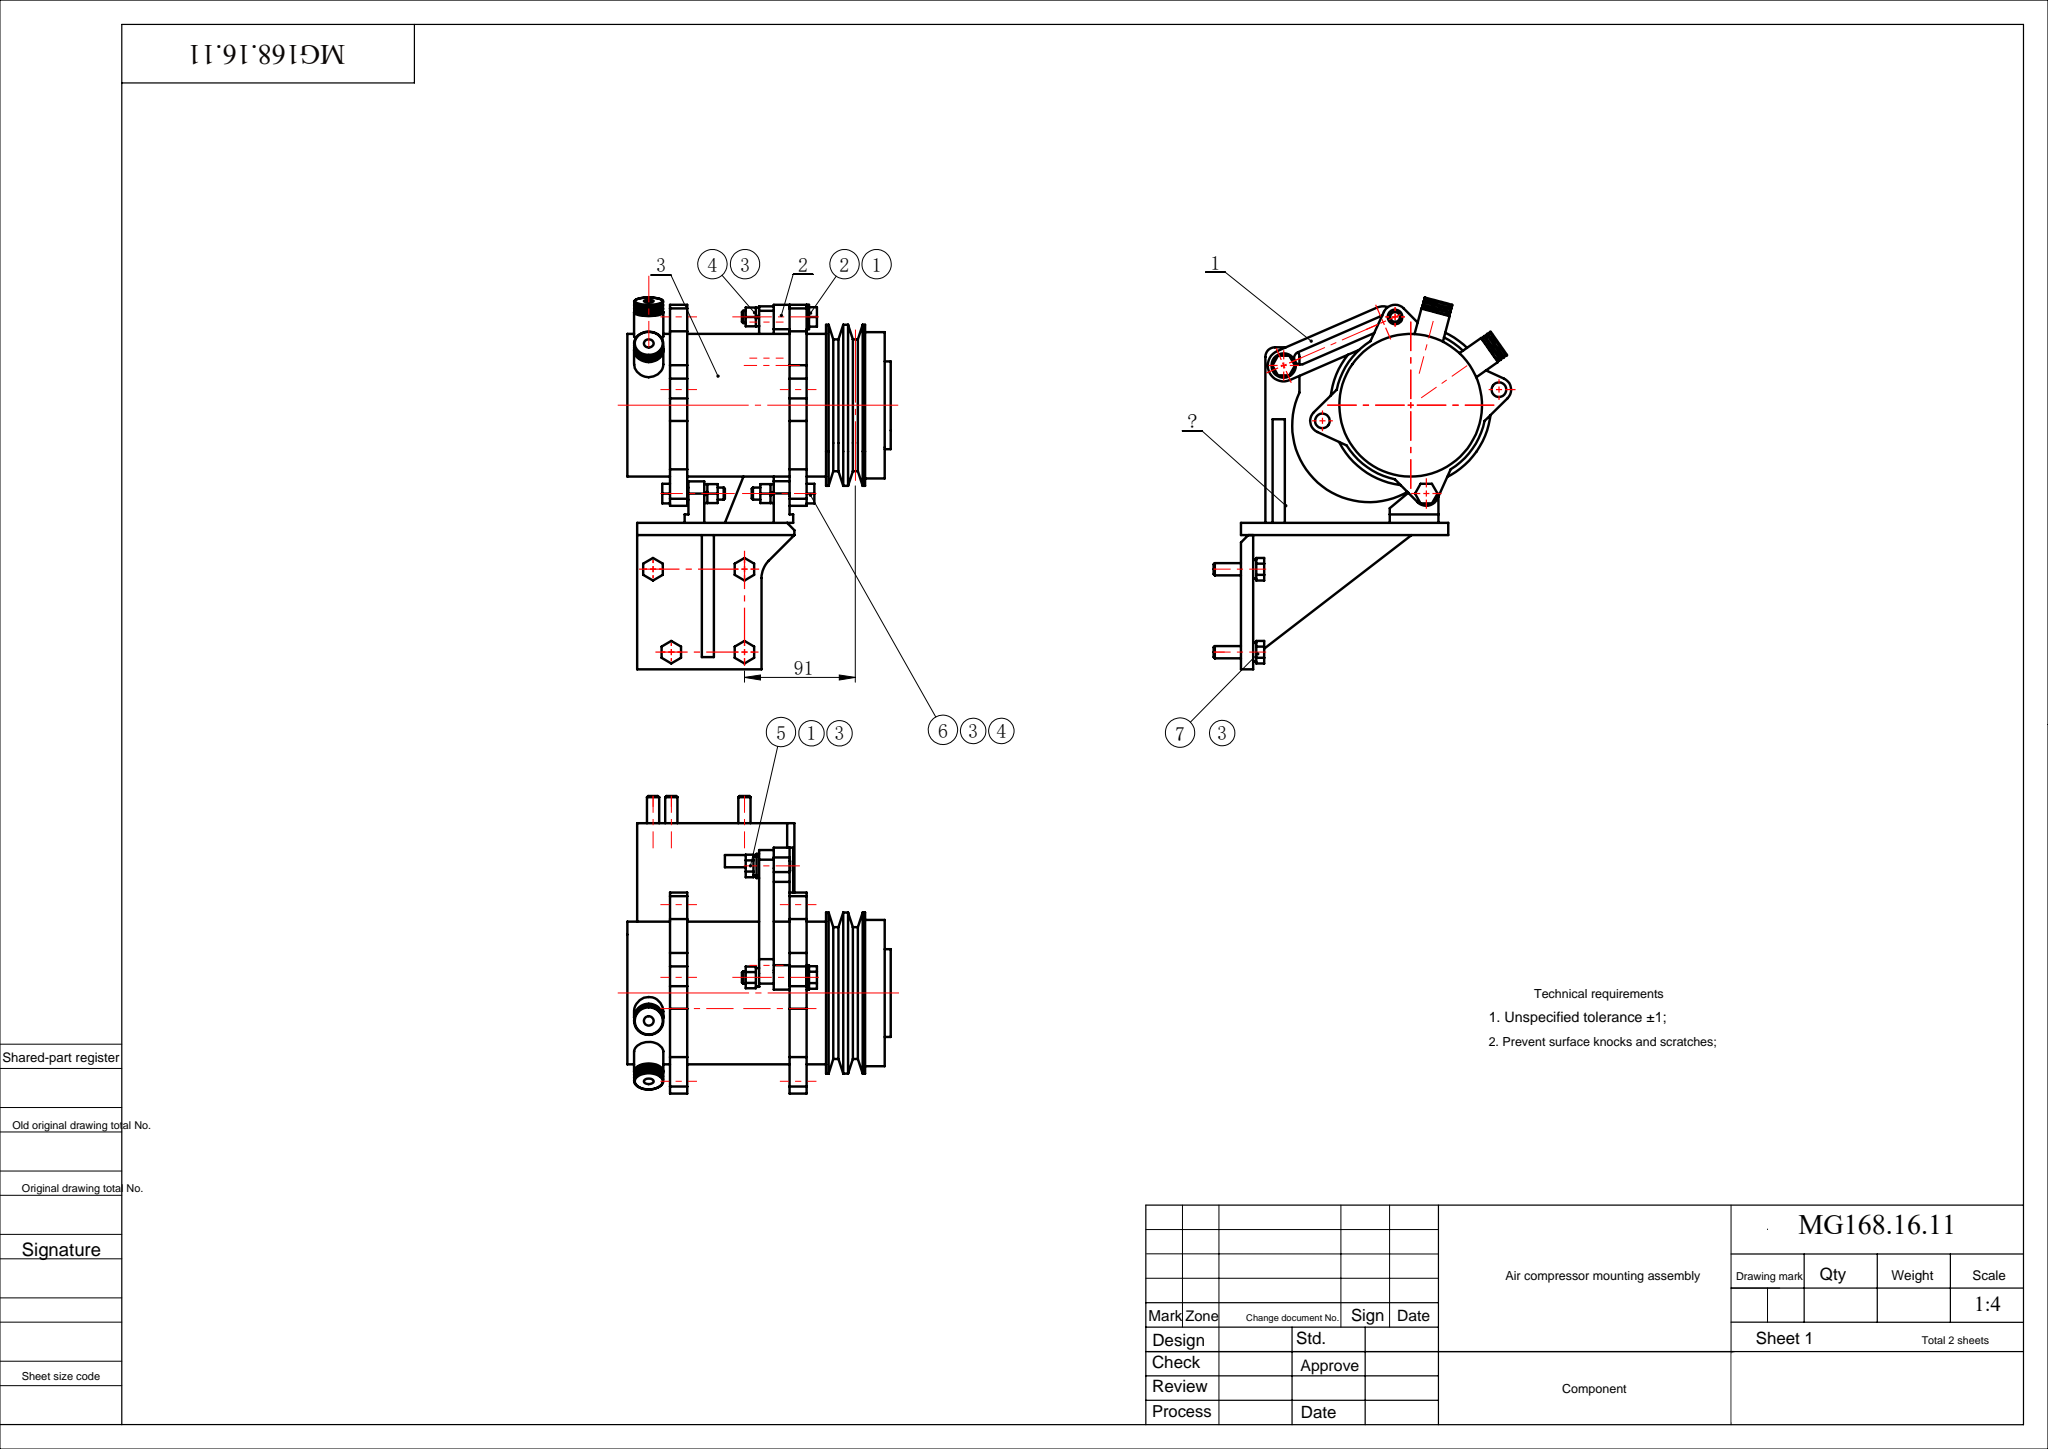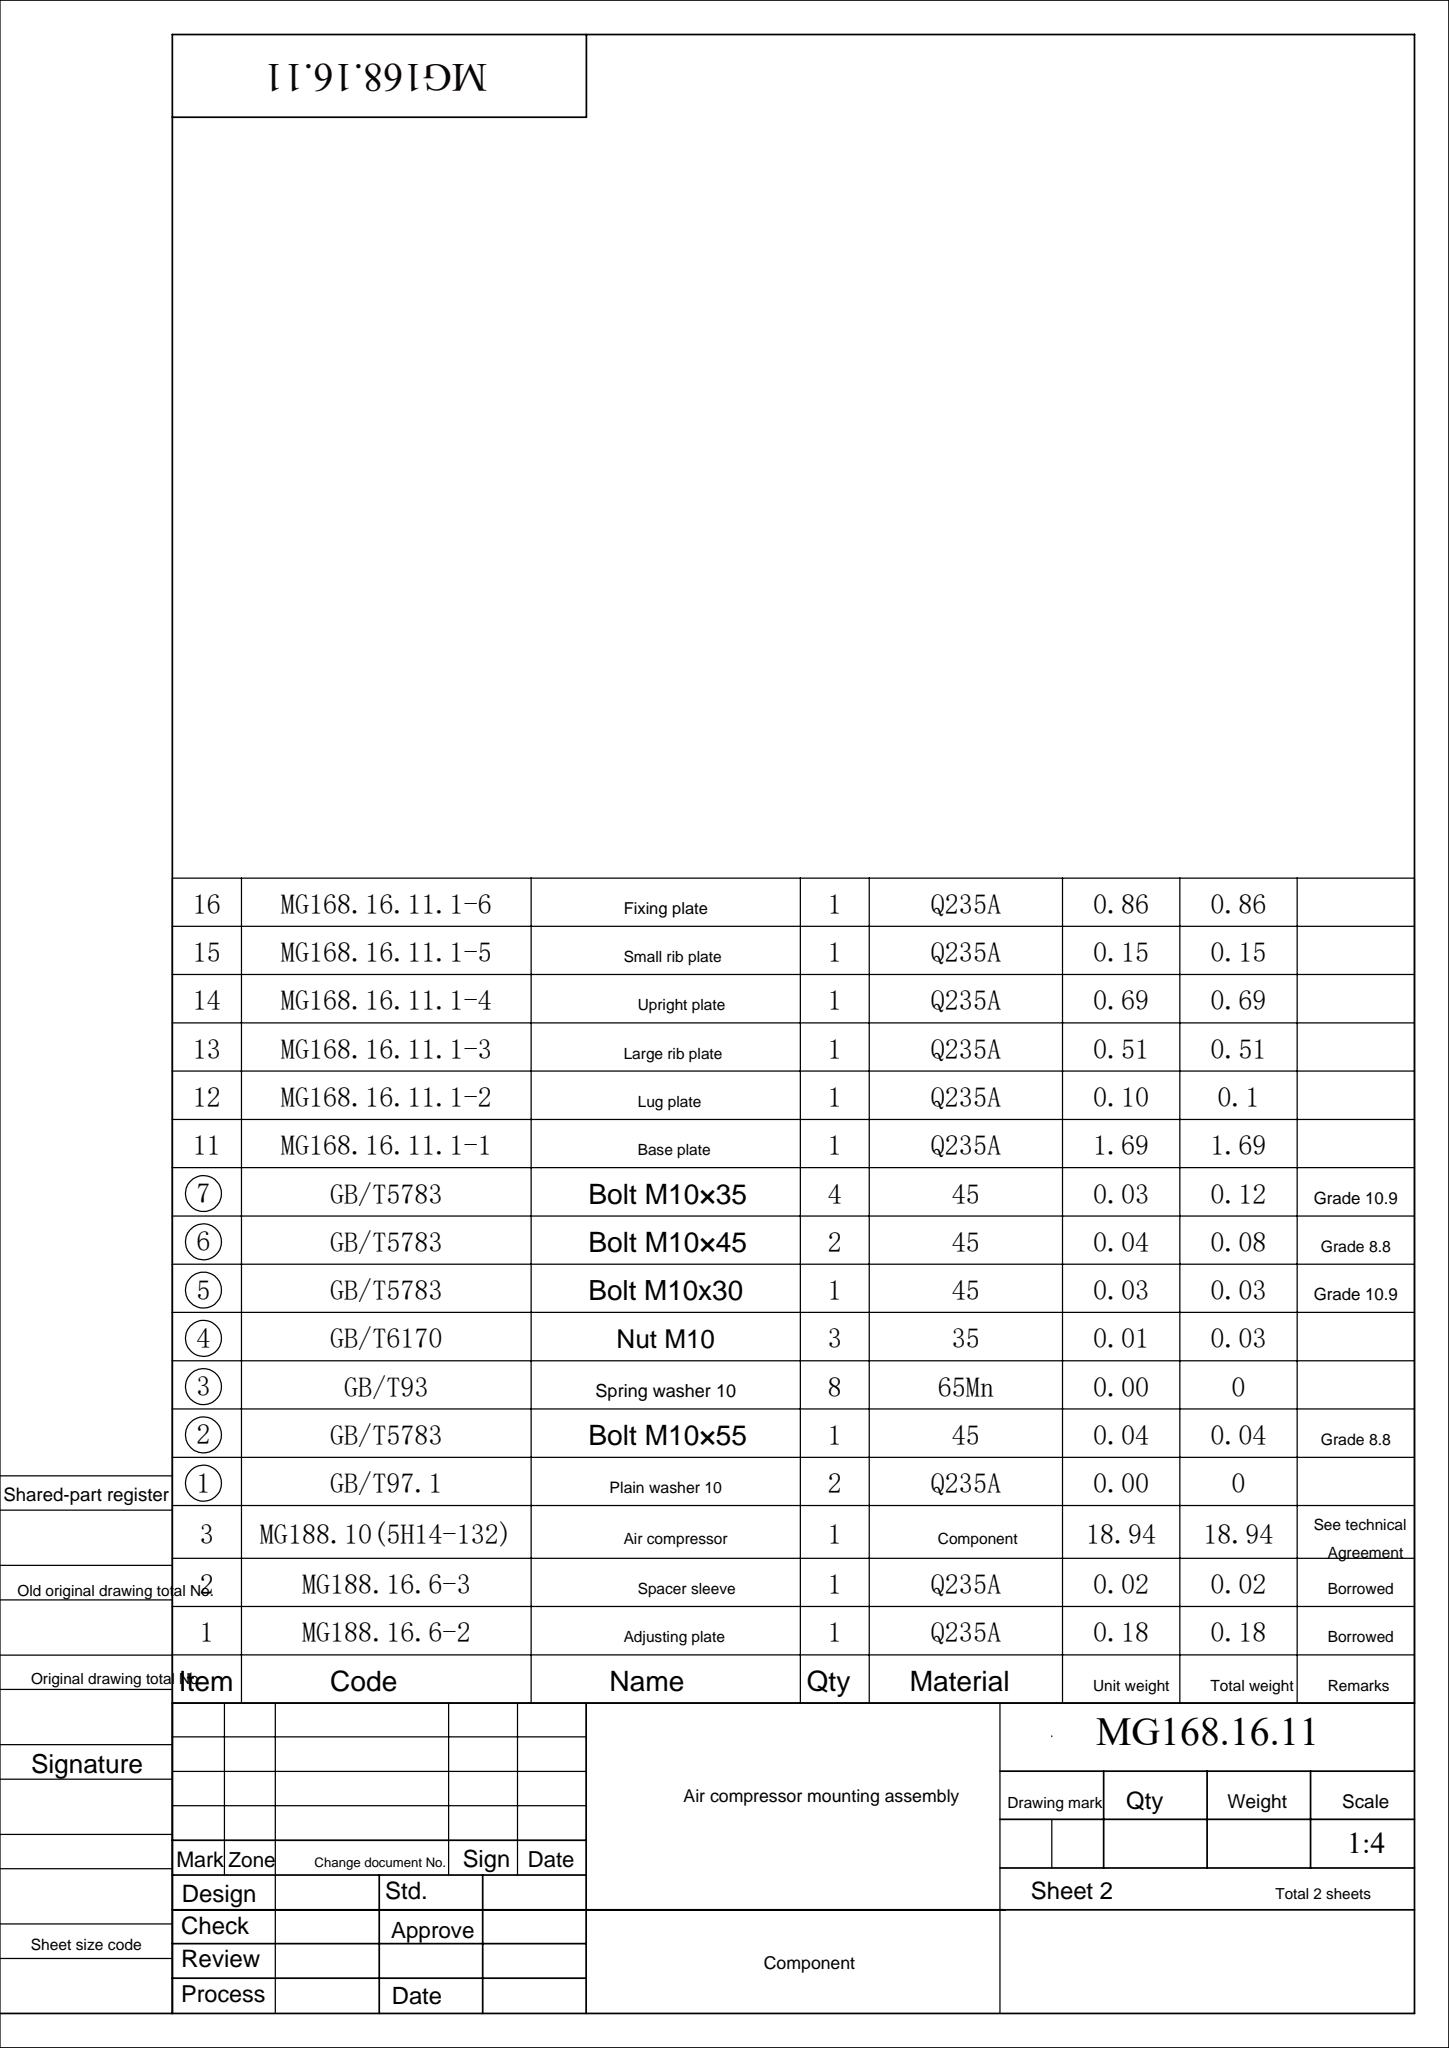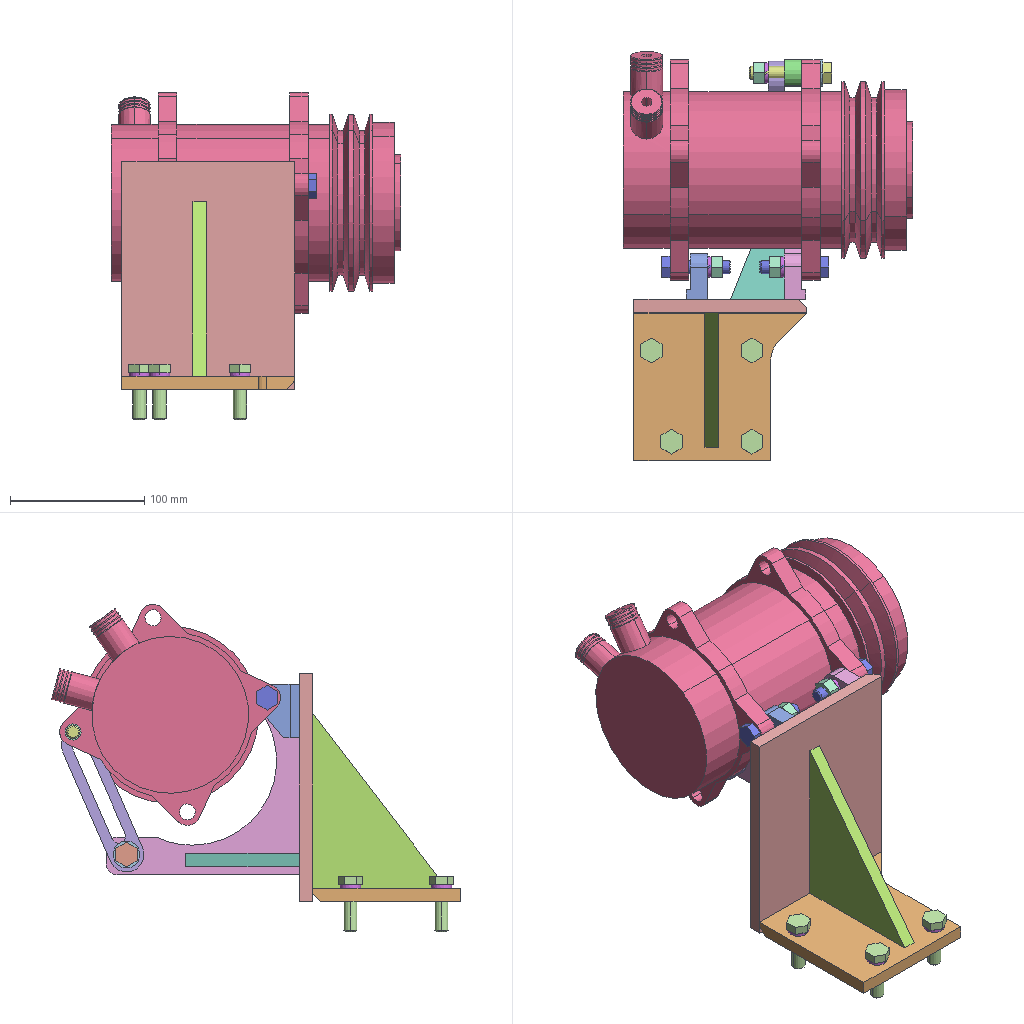Assembly | SolidWorks | 16 different items | 30 placed | box 216 x 305 x 244 mm
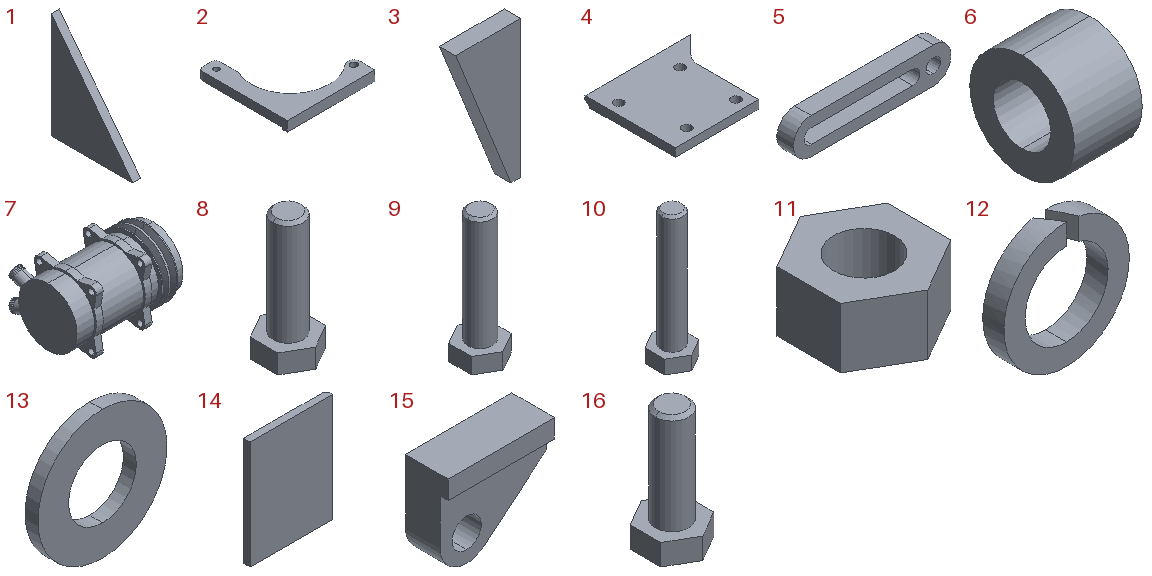Parts list (item | quantity | size | volume | features):
1 | x1 | 10 x 100 x 130 mm | 65000 mm3 | features Extrusion 1
2 | x1 | 142 x 144 x 16 mm | 88798 mm3 | features Extrusion 1, Fillet 1, HoleWzd 1, ICE 1
3 | x1 | 40 x 10 x 85 mm | 19550 mm3 | features Extrusion 1
4 | x1 | 129 x 110 x 10 mm | 109844 mm3 | features Chamfer 1, Extrusion 1, ICE 1
5 | x1 | 115 x 12 x 26 mm | 22737 mm3 | features Extrusion 1
6 | x1 | 13 x 20 x 20 mm | 2849 mm3 | features Extrusion 1
7 | x1 | 216 x 153.032 x 132 mm | 2427701 mm3 | features MirrorPattern 3, ICE 2, Revolution 2, Extrusion 1, LPattern 1
8 | x4 | 16 x 18.475 x 41.4 mm | 4153 mm3 | features Chamfer 1, Extrusion 1, ICE 1, RefAxis 1
9 | x2 | 16 x 18.475 x 51.4 mm | 4939 mm3 | features Chamfer 1, Extrusion 1, ICE 1, RefAxis 1
10 | x1 | 16 x 18.475 x 61.4 mm | 5724 mm3 | features Chamfer 1, Extrusion 1, ICE 1, RefAxis 1
11 | x3 | 15.4 x 17.782 x 8.4 mm | 1249 mm3 | features Extrusion 1, HoleWzd 1, RefAxis 1
12 | x8 | 15.4 x 2.6 x 15.4 mm | 261.639 mm3 | features Extrusion 1, ICE 1
13 | x2 | 20 x 2 x 20 mm | 455.138 mm3 | features Extrusion 1
14 | x1 | 129 x 10 x 170 mm | 216240 mm3 | features Chamfer 1, Extrusion 1
15 | x1 | 40 x 16 x 34 mm | 13215 mm3 | features Extrusion 1, ICE 1
16 | x1 | 16 x 18.475 x 36.4 mm | 3760 mm3 | features Chamfer 1, Extrusion 1, ICE 1, RefAxis 1
Mates (type | each side: item.copy, entity, surface, feature):
Coincident | 5.1 face plane Boss-Extrude1 | 6.1 face plane Boss-Extrude2
Coincident | 5.1 plane | 6.1 plane
Concentric | 6.1 face cylinder Boss-Extrude2 | 7.1 face cylinder Mirror2
Tangent | 5.1 face plane Boss-Extrude1 | 7.1 face cylinder Boss-Extrude1
Coincident | 7.1 face plane Revolve1 | 13.1 face plane Boss-Extrude1
Concentric | 7.1 face cylinder Mirror2 | 13.1 face cylinder Boss-Extrude1
Parallel | 13.1 plane | assembly plane
Concentric | 7.1 face cylinder Mirror2 | 10.1 face cylinder Boss-Extrude2
Coincident | 13.1 face plane Boss-Extrude1 | 10.1 face plane Boss-Extrude1
Coincident | 5.1 face plane Boss-Extrude1 | 12.1 face plane Boss-Extrude1
Concentric | 10.1 face cylinder Boss-Extrude2 | 12.1 face cylinder Boss-Extrude1
Parallel | 10.1 plane | assembly plane
Parallel | 12.1 plane | assembly plane
Parallel | 11.1 plane | assembly plane
Coincident | 12.1 face plane Boss-Extrude1 | 11.1 face plane Boss-Extrude1
Concentric | 10.1 face cylinder Boss-Extrude2 | 11.1 face cylinder M10 Tapped Hole1
Coincident | 5.1 face plane Boss-Extrude1 | 13.2 face plane Boss-Extrude1
Concentric | 5.1 face cylinder Boss-Extrude1 | 13.2 face cylinder Boss-Extrude1
Parallel | 13.2 plane | assembly plane
Coincident | 13.2 face plane Boss-Extrude1 | 12.2 face plane Boss-Extrude1
Concentric | 13.2 edge | 12.2 face cylinder Boss-Extrude1
Parallel | 12.2 plane | assembly plane
Coincident | 12.2 face plane Boss-Extrude1 | 16.1 face plane Boss-Extrude1
Concentric | 12.2 face cylinder Boss-Extrude1 | 16.1 face cylinder Boss-Extrude2
Parallel | 16.1 plane | assembly plane
Coincident | 7.1 face plane Revolve1 | 9.1 face plane Boss-Extrude1
Concentric | 7.1 face cylinder LPattern1 | 9.1 face cylinder Boss-Extrude2
Parallel | 9.1 plane | assembly plane
Concentric | 9.1 face cylinder Boss-Extrude2 | 12.3 face cylinder Boss-Extrude1
Parallel | 12.3 plane | assembly plane
Coincident | 12.3 face plane Boss-Extrude1 | 11.2 face plane Boss-Extrude1
Concentric | 9.1 face cylinder Boss-Extrude2 | 11.2 face cylinder M10 Tapped Hole1
Parallel | assembly plane | 11.2 plane
Concentric | 7.1 face cylinder Mirror3 | 9.2 face cylinder Boss-Extrude2
Coincident | 7.1 face plane Revolve1 | 9.2 face plane Boss-Extrude1
Parallel | 9.2 plane | assembly plane
Concentric | 9.2 face cylinder Boss-Extrude2 | 12.4 face cylinder Boss-Extrude1
Parallel | 12.4 plane | assembly plane
Coincident | 12.4 face plane Boss-Extrude1 | 11.3 face plane Boss-Extrude1
Concentric | 9.2 face cylinder Boss-Extrude2 | 11.3 face cylinder M10 Tapped Hole1
Parallel | 11.3 plane | assembly plane
Parallel | 12.5 plane | assembly plane
Coincident | 12.5 face plane Boss-Extrude1 | 8.1 face plane Boss-Extrude1
Concentric | 8.1 face cylinder Boss-Extrude2 | 12.5 face cylinder Boss-Extrude1
Parallel | 8.1 plane | assembly plane
DistanceDim | 14.1 face plane Boss-Extrude1 | 2.1 face plane Boss-Extrude1
Coincident | 14.1 face plane Boss-Extrude1 | 2.1 face plane Boss-Extrude1
Coincident | 14.1 face plane Boss-Extrude1 | 15.1 face plane Boss-Extrude1
Coincident | 14.1 face plane Boss-Extrude1 | 1.1 face plane Boss-Extrude1
Coincident | 14.1 face plane Boss-Extrude1 | 3.1 face plane Boss-Extrude1
Coincident | 14.1 face plane Boss-Extrude1 | 4.1 face plane Boss-Extrude1
Coincident | 14.1 plane | 4.1 plane
Coincident | 4.1 face plane Boss-Extrude1 | 14.1 face plane Boss-Extrude1
Concentric | 15.1 face cylinder Boss-Extrude1 | 2.1 face cylinder Boss-Extrude1
Coincident | 4.1 face plane Boss-Extrude1 | 1.1 face plane Boss-Extrude1
Coincident | 2.1 face plane Boss-Extrude1 | 3.1 face plane Boss-Extrude1
DistanceDim | 3.1 face plane Boss-Extrude1 | 2.1 face plane Boss-Extrude1
Coincident | 15.1 face plane Boss-Extrude1 | 12.3 face plane Boss-Extrude1
Coincident | 2.1 face plane Boss-Extrude1 | 5.1 face plane Boss-Extrude1
Concentric | 2.1 face cylinder M10 Tapped Hole1 | 5.1 face cylinder Boss-Extrude1
Coincident | 2.1 face plane Boss-Extrude1 | 7.1 face plane Revolve1
Concentric | 2.1 face cylinder Boss-Extrude1 | 7.1 face cylinder Mirror3
Coincident | 2.1 face plane Boss-Extrude1 | 12.4 face plane Boss-Extrude1
Coincident | 4.1 face plane Boss-Extrude1 | 12.5 face plane Boss-Extrude1
Concentric | 12.5 face cylinder Boss-Extrude1 | 4.1 face cylinder Cut-Extrude1